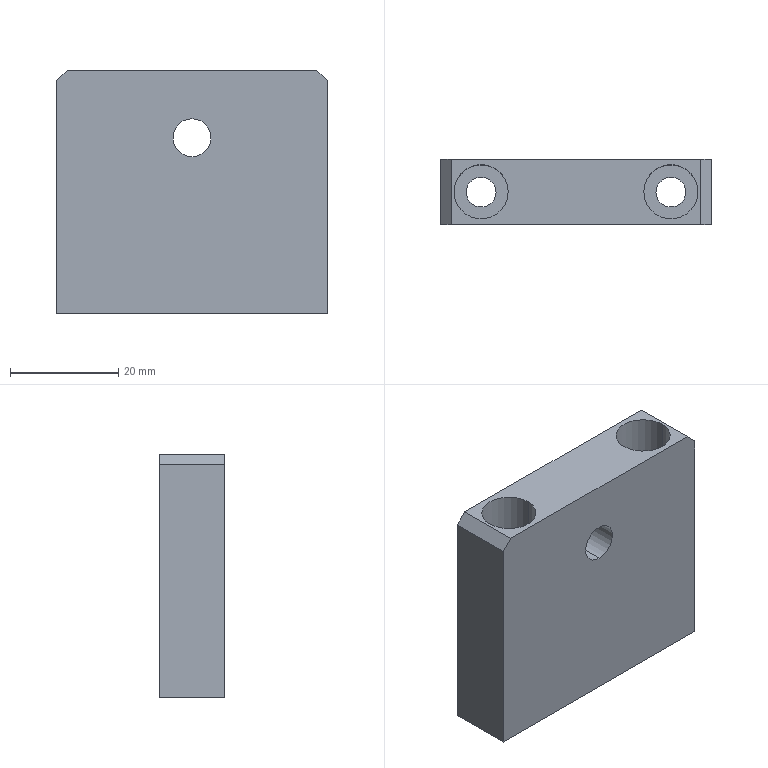Part | SolidWorks | features HoleWzd 2, Chamfer 1, Extrusion 1 | 1 solid | 20 faces | box 50 x 12 x 45 mm | volume 20517 mm3 | cylinder 10 | plane 10 | commonest cylinder face diameters 5.5 x4 10 x4 7 x2
STEP:
#1=CARTESIAN_POINT('',(-22.5,0.,-12.5));
#2=VERTEX_POINT('',#1);
#3=CARTESIAN_POINT('',(-12.5,0.,-12.5));
#4=VERTEX_POINT('',#3);
#5=CARTESIAN_POINT('',(-17.5,0.,-12.5));
#6=DIRECTION('',(0.,0.,1.));
#7=DIRECTION('',(1.,0.,0.));
#8=AXIS2_PLACEMENT_3D('',#5,#6,#7);
#9=CIRCLE('',#8,5.);
#10=EDGE_CURVE('',#2,#4,#9,.T.);
#11=ORIENTED_EDGE('',*,*,#10,.F.);
#12=CARTESIAN_POINT('',(-22.5,0.,22.5));
#13=VERTEX_POINT('',#12);
#14=CARTESIAN_POINT('',(-22.5,0.,22.5));
#15=DIRECTION('',(0.,0.,1.));
#16=VECTOR('',#15,1000.);
#17=LINE('',#14,#16);
#18=EDGE_CURVE('',#2,#13,#17,.T.);
#19=ORIENTED_EDGE('',*,*,#18,.T.);
#20=CARTESIAN_POINT('',(-12.5,0.,22.5));
#21=VERTEX_POINT('',#20);
#22=CARTESIAN_POINT('',(-17.5,0.,22.5));
#23=DIRECTION('',(0.,0.,1.));
#24=DIRECTION('',(1.,0.,0.));
#25=AXIS2_PLACEMENT_3D('',#22,#23,#24);
#26=CIRCLE('',#25,5.);
#27=EDGE_CURVE('',#13,#21,#26,.T.);
#28=ORIENTED_EDGE('',*,*,#27,.T.);
#29=CARTESIAN_POINT('',(-12.5,0.,22.5));
#30=DIRECTION('',(0.,0.,1.));
#31=VECTOR('',#30,1000.);
#32=LINE('',#29,#31);
#33=EDGE_CURVE('',#4,#21,#32,.T.);
#34=ORIENTED_EDGE('',*,*,#33,.F.);
#35=EDGE_LOOP('',(#11,#19,#28,#34));
#36=FACE_OUTER_BOUND('',#35,.T.);
#37=CARTESIAN_POINT('',(-17.5,0.,22.5));
#38=DIRECTION('',(0.,0.,1.));
#39=DIRECTION('',(1.,0.,0.));
#40=AXIS2_PLACEMENT_3D('',#37,#38,#39);
#41=CYLINDRICAL_SURFACE('',#40,5.);
#42=ADVANCED_FACE('',(#36),#41,.F.);
#43=CARTESIAN_POINT('',(-20.25,0.,-22.5));
#44=VERTEX_POINT('',#43);
#45=CARTESIAN_POINT('',(-14.75,0.,-22.5));
#46=VERTEX_POINT('',#45);
#47=CARTESIAN_POINT('',(-17.5,0.,-22.5));
#48=DIRECTION('',(0.,0.,1.));
#49=DIRECTION('',(1.,0.,0.));
#50=AXIS2_PLACEMENT_3D('',#47,#48,#49);
#51=CIRCLE('',#50,2.75);
#52=EDGE_CURVE('',#44,#46,#51,.T.);
#53=ORIENTED_EDGE('',*,*,#52,.F.);
#54=CARTESIAN_POINT('',(-20.25,0.,-12.5));
#55=VERTEX_POINT('',#54);
#56=CARTESIAN_POINT('',(-20.25,0.,22.5));
#57=DIRECTION('',(0.,0.,1.));
#58=VECTOR('',#57,1000.);
#59=LINE('',#56,#58);
#60=EDGE_CURVE('',#44,#55,#59,.T.);
#61=ORIENTED_EDGE('',*,*,#60,.T.);
#62=CARTESIAN_POINT('',(-14.75,0.,-12.5));
#63=VERTEX_POINT('',#62);
#64=CARTESIAN_POINT('',(-17.5,0.,-12.5));
#65=DIRECTION('',(0.,0.,1.));
#66=DIRECTION('',(1.,0.,0.));
#67=AXIS2_PLACEMENT_3D('',#64,#65,#66);
#68=CIRCLE('',#67,2.75);
#69=EDGE_CURVE('',#55,#63,#68,.T.);
#70=ORIENTED_EDGE('',*,*,#69,.T.);
#71=CARTESIAN_POINT('',(-14.75,0.,22.5));
#72=DIRECTION('',(0.,0.,1.));
#73=VECTOR('',#72,1000.);
#74=LINE('',#71,#73);
#75=EDGE_CURVE('',#46,#63,#74,.T.);
#76=ORIENTED_EDGE('',*,*,#75,.F.);
#77=EDGE_LOOP('',(#53,#61,#70,#76));
#78=FACE_OUTER_BOUND('',#77,.T.);
#79=CARTESIAN_POINT('',(-17.5,0.,22.5));
#80=DIRECTION('',(0.,0.,1.));
#81=DIRECTION('',(1.,0.,0.));
#82=AXIS2_PLACEMENT_3D('',#79,#80,#81);
#83=CYLINDRICAL_SURFACE('',#82,2.75);
#84=ADVANCED_FACE('',(#78),#83,.F.);
#85=CARTESIAN_POINT('',(12.5,0.,-12.5));
#86=VERTEX_POINT('',#85);
#87=CARTESIAN_POINT('',(22.5,0.,-12.5));
#88=VERTEX_POINT('',#87);
#89=CARTESIAN_POINT('',(17.5,0.,-12.5));
#90=DIRECTION('',(0.,0.,1.));
#91=DIRECTION('',(1.,0.,0.));
#92=AXIS2_PLACEMENT_3D('',#89,#90,#91);
#93=CIRCLE('',#92,5.);
#94=EDGE_CURVE('',#86,#88,#93,.T.);
#95=ORIENTED_EDGE('',*,*,#94,.F.);
#96=CARTESIAN_POINT('',(12.5,0.,22.5));
#97=VERTEX_POINT('',#96);
#98=CARTESIAN_POINT('',(12.5,0.,22.5));
#99=DIRECTION('',(0.,0.,1.));
#100=VECTOR('',#99,1000.);
#101=LINE('',#98,#100);
#102=EDGE_CURVE('',#86,#97,#101,.T.);
#103=ORIENTED_EDGE('',*,*,#102,.T.);
#104=CARTESIAN_POINT('',(22.5,0.,22.5));
#105=VERTEX_POINT('',#104);
#106=CARTESIAN_POINT('',(17.5,0.,22.5));
#107=DIRECTION('',(0.,0.,1.));
#108=DIRECTION('',(1.,0.,0.));
#109=AXIS2_PLACEMENT_3D('',#106,#107,#108);
#110=CIRCLE('',#109,5.);
#111=EDGE_CURVE('',#97,#105,#110,.T.);
#112=ORIENTED_EDGE('',*,*,#111,.T.);
#113=CARTESIAN_POINT('',(22.5,0.,22.5));
#114=DIRECTION('',(0.,0.,1.));
#115=VECTOR('',#114,1000.);
#116=LINE('',#113,#115);
#117=EDGE_CURVE('',#88,#105,#116,.T.);
#118=ORIENTED_EDGE('',*,*,#117,.F.);
#119=EDGE_LOOP('',(#95,#103,#112,#118));
#120=FACE_OUTER_BOUND('',#119,.T.);
#121=CARTESIAN_POINT('',(17.5,0.,22.5));
#122=DIRECTION('',(0.,0.,1.));
#123=DIRECTION('',(1.,0.,0.));
#124=AXIS2_PLACEMENT_3D('',#121,#122,#123);
#125=CYLINDRICAL_SURFACE('',#124,5.);
#126=ADVANCED_FACE('',(#120),#125,.F.);
#127=CARTESIAN_POINT('',(14.75,0.,-22.5));
#128=VERTEX_POINT('',#127);
#129=CARTESIAN_POINT('',(20.25,0.,-22.5));
#130=VERTEX_POINT('',#129);
#131=CARTESIAN_POINT('',(17.5,0.,-22.5));
#132=DIRECTION('',(0.,0.,1.));
#133=DIRECTION('',(1.,0.,0.));
#134=AXIS2_PLACEMENT_3D('',#131,#132,#133);
#135=CIRCLE('',#134,2.75);
#136=EDGE_CURVE('',#128,#130,#135,.T.);
#137=ORIENTED_EDGE('',*,*,#136,.F.);
#138=CARTESIAN_POINT('',(14.75,0.,-12.5));
#139=VERTEX_POINT('',#138);
#140=CARTESIAN_POINT('',(14.75,0.,22.5));
#141=DIRECTION('',(0.,0.,1.));
#142=VECTOR('',#141,1000.);
#143=LINE('',#140,#142);
#144=EDGE_CURVE('',#128,#139,#143,.T.);
#145=ORIENTED_EDGE('',*,*,#144,.T.);
#146=CARTESIAN_POINT('',(20.25,0.,-12.5));
#147=VERTEX_POINT('',#146);
#148=CARTESIAN_POINT('',(17.5,0.,-12.5));
#149=DIRECTION('',(0.,0.,1.));
#150=DIRECTION('',(1.,0.,0.));
#151=AXIS2_PLACEMENT_3D('',#148,#149,#150);
#152=CIRCLE('',#151,2.75);
#153=EDGE_CURVE('',#139,#147,#152,.T.);
#154=ORIENTED_EDGE('',*,*,#153,.T.);
#155=CARTESIAN_POINT('',(20.25,0.,22.5));
#156=DIRECTION('',(0.,0.,1.));
#157=VECTOR('',#156,1000.);
#158=LINE('',#155,#157);
#159=EDGE_CURVE('',#130,#147,#158,.T.);
#160=ORIENTED_EDGE('',*,*,#159,.F.);
#161=EDGE_LOOP('',(#137,#145,#154,#160));
#162=FACE_OUTER_BOUND('',#161,.T.);
#163=CARTESIAN_POINT('',(17.5,0.,22.5));
#164=DIRECTION('',(0.,0.,1.));
#165=DIRECTION('',(1.,0.,0.));
#166=AXIS2_PLACEMENT_3D('',#163,#164,#165);
#167=CYLINDRICAL_SURFACE('',#166,2.75);
#168=ADVANCED_FACE('',(#162),#167,.F.);
#169=CARTESIAN_POINT('',(0.,-6.,6.5));
#170=VERTEX_POINT('',#169);
#171=CARTESIAN_POINT('',(0.,-6.,13.5));
#172=VERTEX_POINT('',#171);
#173=CARTESIAN_POINT('',(0.,-6.,10.));
#174=DIRECTION('',(0.,1.,0.));
#175=DIRECTION('',(-1.,0.,0.));
#176=AXIS2_PLACEMENT_3D('',#173,#174,#175);
#177=CIRCLE('',#176,3.5);
#178=EDGE_CURVE('',#170,#172,#177,.T.);
#179=ORIENTED_EDGE('',*,*,#178,.F.);
#180=CARTESIAN_POINT('',(0.,6.,6.5));
#181=VERTEX_POINT('',#180);
#182=CARTESIAN_POINT('',(0.,6.,6.5));
#183=DIRECTION('',(0.,1.,0.));
#184=VECTOR('',#183,1000.);
#185=LINE('',#182,#184);
#186=EDGE_CURVE('',#170,#181,#185,.T.);
#187=ORIENTED_EDGE('',*,*,#186,.T.);
#188=CARTESIAN_POINT('',(0.,6.,13.5));
#189=VERTEX_POINT('',#188);
#190=CARTESIAN_POINT('',(0.,6.,10.));
#191=DIRECTION('',(0.,1.,0.));
#192=DIRECTION('',(0.,0.,1.));
#193=AXIS2_PLACEMENT_3D('',#190,#191,#192);
#194=CIRCLE('',#193,3.5);
#195=EDGE_CURVE('',#181,#189,#194,.T.);
#196=ORIENTED_EDGE('',*,*,#195,.T.);
#197=CARTESIAN_POINT('',(0.,6.,13.5));
#198=DIRECTION('',(0.,1.,0.));
#199=VECTOR('',#198,1000.);
#200=LINE('',#197,#199);
#201=EDGE_CURVE('',#172,#189,#200,.T.);
#202=ORIENTED_EDGE('',*,*,#201,.F.);
#203=EDGE_LOOP('',(#179,#187,#196,#202));
#204=FACE_OUTER_BOUND('',#203,.T.);
#205=CARTESIAN_POINT('',(0.,6.,10.));
#206=DIRECTION('',(0.,1.,0.));
#207=DIRECTION('',(0.,0.,1.));
#208=AXIS2_PLACEMENT_3D('',#205,#206,#207);
#209=CYLINDRICAL_SURFACE('',#208,3.5);
#210=ADVANCED_FACE('',(#204),#209,.F.);
#211=CARTESIAN_POINT('',(-25.,6.,20.5));
#212=VERTEX_POINT('',#211);
#213=CARTESIAN_POINT('',(-25.,6.,-22.5));
#214=VERTEX_POINT('',#213);
#215=CARTESIAN_POINT('',(-25.,6.,22.5));
#216=DIRECTION('',(0.,0.,-1.));
#217=VECTOR('',#216,1000.);
#218=LINE('',#215,#217);
#219=EDGE_CURVE('',#212,#214,#218,.T.);
#220=ORIENTED_EDGE('',*,*,#219,.F.);
#221=CARTESIAN_POINT('',(-23.,6.,22.5));
#222=VERTEX_POINT('',#221);
#223=CARTESIAN_POINT('',(-23.,6.,22.5));
#224=DIRECTION('',(0.7071,0.,0.7071));
#225=VECTOR('',#224,1000.);
#226=LINE('',#223,#225);
#227=EDGE_CURVE('',#212,#222,#226,.T.);
#228=ORIENTED_EDGE('',*,*,#227,.T.);
#229=CARTESIAN_POINT('',(23.,6.,22.5));
#230=VERTEX_POINT('',#229);
#231=CARTESIAN_POINT('',(25.,6.,22.5));
#232=DIRECTION('',(-1.,0.,0.));
#233=VECTOR('',#232,1000.);
#234=LINE('',#231,#233);
#235=EDGE_CURVE('',#230,#222,#234,.T.);
#236=ORIENTED_EDGE('',*,*,#235,.F.);
#237=CARTESIAN_POINT('',(25.,6.,20.5));
#238=VERTEX_POINT('',#237);
#239=CARTESIAN_POINT('',(23.,6.,22.5));
#240=DIRECTION('',(0.7071,0.,-0.7071));
#241=VECTOR('',#240,1000.);
#242=LINE('',#239,#241);
#243=EDGE_CURVE('',#230,#238,#242,.T.);
#244=ORIENTED_EDGE('',*,*,#243,.T.);
#245=CARTESIAN_POINT('',(25.,6.,-22.5));
#246=VERTEX_POINT('',#245);
#247=CARTESIAN_POINT('',(25.,6.,22.5));
#248=DIRECTION('',(0.,0.,-1.));
#249=VECTOR('',#248,1000.);
#250=LINE('',#247,#249);
#251=EDGE_CURVE('',#238,#246,#250,.T.);
#252=ORIENTED_EDGE('',*,*,#251,.T.);
#253=CARTESIAN_POINT('',(25.,6.,-22.5));
#254=DIRECTION('',(-1.,0.,0.));
#255=VECTOR('',#254,1000.);
#256=LINE('',#253,#255);
#257=EDGE_CURVE('',#246,#214,#256,.T.);
#258=ORIENTED_EDGE('',*,*,#257,.T.);
#259=EDGE_LOOP('',(#220,#228,#236,#244,#252,#258));
#260=FACE_OUTER_BOUND('',#259,.T.);
#261=CARTESIAN_POINT('',(0.,6.,10.));
#262=DIRECTION('',(0.,1.,0.));
#263=DIRECTION('',(0.,0.,1.));
#264=AXIS2_PLACEMENT_3D('',#261,#262,#263);
#265=CIRCLE('',#264,3.5);
#266=EDGE_CURVE('',#189,#181,#265,.T.);
#267=ORIENTED_EDGE('',*,*,#266,.F.);
#268=ORIENTED_EDGE('',*,*,#195,.F.);
#269=EDGE_LOOP('',(#267,#268));
#270=FACE_BOUND('',#269,.T.);
#271=CARTESIAN_POINT('',(25.,6.,22.5));
#272=DIRECTION('',(0.,-1.,0.));
#273=DIRECTION('',(1.,0.,0.));
#274=AXIS2_PLACEMENT_3D('',#271,#272,#273);
#275=PLANE('',#274);
#276=ADVANCED_FACE('',(#260,#270),#275,.F.);
#277=CARTESIAN_POINT('',(-25.,-6.,20.5));
#278=VERTEX_POINT('',#277);
#279=CARTESIAN_POINT('',(-25.,-6.,-22.5));
#280=VERTEX_POINT('',#279);
#281=CARTESIAN_POINT('',(-25.,-6.,22.5));
#282=DIRECTION('',(0.,0.,-1.));
#283=VECTOR('',#282,1000.);
#284=LINE('',#281,#283);
#285=EDGE_CURVE('',#278,#280,#284,.T.);
#286=ORIENTED_EDGE('',*,*,#285,.F.);
#287=CARTESIAN_POINT('',(-25.,6.,20.5));
#288=DIRECTION('',(0.,1.,0.));
#289=VECTOR('',#288,1000.);
#290=LINE('',#287,#289);
#291=EDGE_CURVE('',#278,#212,#290,.T.);
#292=ORIENTED_EDGE('',*,*,#291,.T.);
#293=ORIENTED_EDGE('',*,*,#219,.T.);
#294=CARTESIAN_POINT('',(-25.,-6.,-22.5));
#295=DIRECTION('',(0.,-1.,0.));
#296=VECTOR('',#295,1000.);
#297=LINE('',#294,#296);
#298=EDGE_CURVE('',#214,#280,#297,.T.);
#299=ORIENTED_EDGE('',*,*,#298,.T.);
#300=EDGE_LOOP('',(#286,#292,#293,#299));
#301=FACE_OUTER_BOUND('',#300,.T.);
#302=CARTESIAN_POINT('',(-25.,-6.,22.5));
#303=DIRECTION('',(1.,0.,0.));
#304=DIRECTION('',(0.,0.,-1.));
#305=AXIS2_PLACEMENT_3D('',#302,#303,#304);
#306=PLANE('',#305);
#307=ADVANCED_FACE('',(#301),#306,.F.);
#308=CARTESIAN_POINT('',(0.,-6.,10.));
#309=DIRECTION('',(0.,1.,0.));
#310=DIRECTION('',(-1.,0.,0.));
#311=AXIS2_PLACEMENT_3D('',#308,#309,#310);
#312=CIRCLE('',#311,3.5);
#313=EDGE_CURVE('',#172,#170,#312,.T.);
#314=ORIENTED_EDGE('',*,*,#313,.T.);
#315=ORIENTED_EDGE('',*,*,#178,.T.);
#316=EDGE_LOOP('',(#314,#315));
#317=FACE_BOUND('',#316,.T.);
#318=CARTESIAN_POINT('',(-23.,-6.,22.5));
#319=VERTEX_POINT('',#318);
#320=CARTESIAN_POINT('',(23.,-6.,22.5));
#321=VERTEX_POINT('',#320);
#322=CARTESIAN_POINT('',(25.,-6.,22.5));
#323=DIRECTION('',(1.,0.,0.));
#324=VECTOR('',#323,1000.);
#325=LINE('',#322,#324);
#326=EDGE_CURVE('',#319,#321,#325,.T.);
#327=ORIENTED_EDGE('',*,*,#326,.F.);
#328=CARTESIAN_POINT('',(-23.,-6.,22.5));
#329=DIRECTION('',(-0.7071,0.,-0.7071));
#330=VECTOR('',#329,1000.);
#331=LINE('',#328,#330);
#332=EDGE_CURVE('',#319,#278,#331,.T.);
#333=ORIENTED_EDGE('',*,*,#332,.T.);
#334=ORIENTED_EDGE('',*,*,#285,.T.);
#335=CARTESIAN_POINT('',(25.,-6.,-22.5));
#336=VERTEX_POINT('',#335);
#337=CARTESIAN_POINT('',(25.,-6.,-22.5));
#338=DIRECTION('',(1.,0.,0.));
#339=VECTOR('',#338,1000.);
#340=LINE('',#337,#339);
#341=EDGE_CURVE('',#280,#336,#340,.T.);
#342=ORIENTED_EDGE('',*,*,#341,.T.);
#343=CARTESIAN_POINT('',(25.,-6.,20.5));
#344=VERTEX_POINT('',#343);
#345=CARTESIAN_POINT('',(25.,-6.,22.5));
#346=DIRECTION('',(0.,0.,-1.));
#347=VECTOR('',#346,1000.);
#348=LINE('',#345,#347);
#349=EDGE_CURVE('',#344,#336,#348,.T.);
#350=ORIENTED_EDGE('',*,*,#349,.F.);
#351=CARTESIAN_POINT('',(23.,-6.,22.5));
#352=DIRECTION('',(-0.7071,0.,0.7071));
#353=VECTOR('',#352,1000.);
#354=LINE('',#351,#353);
#355=EDGE_CURVE('',#344,#321,#354,.T.);
#356=ORIENTED_EDGE('',*,*,#355,.T.);
#357=EDGE_LOOP('',(#327,#333,#334,#342,#350,#356));
#358=FACE_OUTER_BOUND('',#357,.T.);
#359=CARTESIAN_POINT('',(25.,-6.,22.5));
#360=DIRECTION('',(0.,1.,0.));
#361=DIRECTION('',(-1.,0.,0.));
#362=AXIS2_PLACEMENT_3D('',#359,#360,#361);
#363=PLANE('',#362);
#364=ADVANCED_FACE('',(#317,#358),#363,.F.);
#365=ORIENTED_EDGE('',*,*,#251,.F.);
#366=CARTESIAN_POINT('',(25.,-6.,20.5));
#367=DIRECTION('',(0.,-1.,0.));
#368=VECTOR('',#367,1000.);
#369=LINE('',#366,#368);
#370=EDGE_CURVE('',#238,#344,#369,.T.);
#371=ORIENTED_EDGE('',*,*,#370,.T.);
#372=ORIENTED_EDGE('',*,*,#349,.T.);
#373=CARTESIAN_POINT('',(25.,-6.,-22.5));
#374=DIRECTION('',(0.,1.,0.));
#375=VECTOR('',#374,1000.);
#376=LINE('',#373,#375);
#377=EDGE_CURVE('',#336,#246,#376,.T.);
#378=ORIENTED_EDGE('',*,*,#377,.T.);
#379=EDGE_LOOP('',(#365,#371,#372,#378));
#380=FACE_OUTER_BOUND('',#379,.T.);
#381=CARTESIAN_POINT('',(25.,-6.,22.5));
#382=DIRECTION('',(-1.,0.,0.));
#383=DIRECTION('',(0.,0.,1.));
#384=AXIS2_PLACEMENT_3D('',#381,#382,#383);
#385=PLANE('',#384);
#386=ADVANCED_FACE('',(#380),#385,.F.);
#387=CARTESIAN_POINT('',(-17.5,0.,22.5));
#388=DIRECTION('',(0.,0.,1.));
#389=DIRECTION('',(1.,0.,0.));
#390=AXIS2_PLACEMENT_3D('',#387,#388,#389);
#391=CIRCLE('',#390,5.);
#392=EDGE_CURVE('',#21,#13,#391,.T.);
#393=ORIENTED_EDGE('',*,*,#392,.F.);
#394=ORIENTED_EDGE('',*,*,#27,.F.);
#395=EDGE_LOOP('',(#393,#394));
#396=FACE_BOUND('',#395,.T.);
#397=CARTESIAN_POINT('',(17.5,0.,22.5));
#398=DIRECTION('',(0.,0.,1.));
#399=DIRECTION('',(1.,0.,0.));
#400=AXIS2_PLACEMENT_3D('',#397,#398,#399);
#401=CIRCLE('',#400,5.);
#402=EDGE_CURVE('',#105,#97,#401,.T.);
#403=ORIENTED_EDGE('',*,*,#402,.F.);
#404=ORIENTED_EDGE('',*,*,#111,.F.);
#405=EDGE_LOOP('',(#403,#404));
#406=FACE_BOUND('',#405,.T.);
#407=ORIENTED_EDGE('',*,*,#235,.T.);
#408=CARTESIAN_POINT('',(-23.,-6.,22.5));
#409=DIRECTION('',(0.,-1.,0.));
#410=VECTOR('',#409,1000.);
#411=LINE('',#408,#410);
#412=EDGE_CURVE('',#222,#319,#411,.T.);
#413=ORIENTED_EDGE('',*,*,#412,.T.);
#414=ORIENTED_EDGE('',*,*,#326,.T.);
#415=CARTESIAN_POINT('',(23.,6.,22.5));
#416=DIRECTION('',(0.,1.,0.));
#417=VECTOR('',#416,1000.);
#418=LINE('',#415,#417);
#419=EDGE_CURVE('',#321,#230,#418,.T.);
#420=ORIENTED_EDGE('',*,*,#419,.T.);
#421=EDGE_LOOP('',(#407,#413,#414,#420));
#422=FACE_OUTER_BOUND('',#421,.T.);
#423=CARTESIAN_POINT('',(0.,0.,22.5));
#424=DIRECTION('',(0.,0.,1.));
#425=DIRECTION('',(1.,0.,0.));
#426=AXIS2_PLACEMENT_3D('',#423,#424,#425);
#427=PLANE('',#426);
#428=ADVANCED_FACE('',(#396,#406,#422),#427,.T.);
#429=CARTESIAN_POINT('',(-17.5,0.,-22.5));
#430=DIRECTION('',(0.,0.,1.));
#431=DIRECTION('',(1.,0.,0.));
#432=AXIS2_PLACEMENT_3D('',#429,#430,#431);
#433=CIRCLE('',#432,2.75);
#434=EDGE_CURVE('',#46,#44,#433,.T.);
#435=ORIENTED_EDGE('',*,*,#434,.T.);
#436=ORIENTED_EDGE('',*,*,#52,.T.);
#437=EDGE_LOOP('',(#435,#436));
#438=FACE_BOUND('',#437,.T.);
#439=CARTESIAN_POINT('',(17.5,0.,-22.5));
#440=DIRECTION('',(0.,0.,1.));
#441=DIRECTION('',(1.,0.,0.));
#442=AXIS2_PLACEMENT_3D('',#439,#440,#441);
#443=CIRCLE('',#442,2.75);
#444=EDGE_CURVE('',#130,#128,#443,.T.);
#445=ORIENTED_EDGE('',*,*,#444,.T.);
#446=ORIENTED_EDGE('',*,*,#136,.T.);
#447=EDGE_LOOP('',(#445,#446));
#448=FACE_BOUND('',#447,.T.);
#449=ORIENTED_EDGE('',*,*,#298,.F.);
#450=ORIENTED_EDGE('',*,*,#257,.F.);
#451=ORIENTED_EDGE('',*,*,#377,.F.);
#452=ORIENTED_EDGE('',*,*,#341,.F.);
#453=EDGE_LOOP('',(#449,#450,#451,#452));
#454=FACE_OUTER_BOUND('',#453,.T.);
#455=CARTESIAN_POINT('',(0.,0.,-22.5));
#456=DIRECTION('',(0.,0.,1.));
#457=DIRECTION('',(1.,0.,0.));
#458=AXIS2_PLACEMENT_3D('',#455,#456,#457);
#459=PLANE('',#458);
#460=ADVANCED_FACE('',(#438,#448,#454),#459,.F.);
#461=ORIENTED_EDGE('',*,*,#186,.F.);
#462=ORIENTED_EDGE('',*,*,#313,.F.);
#463=ORIENTED_EDGE('',*,*,#201,.T.);
#464=ORIENTED_EDGE('',*,*,#266,.T.);
#465=EDGE_LOOP('',(#461,#462,#463,#464));
#466=FACE_OUTER_BOUND('',#465,.T.);
#467=CARTESIAN_POINT('',(0.,6.,10.));
#468=DIRECTION('',(0.,1.,0.));
#469=DIRECTION('',(0.,0.,1.));
#470=AXIS2_PLACEMENT_3D('',#467,#468,#469);
#471=CYLINDRICAL_SURFACE('',#470,3.5);
#472=ADVANCED_FACE('',(#466),#471,.F.);
#473=ORIENTED_EDGE('',*,*,#144,.F.);
#474=ORIENTED_EDGE('',*,*,#444,.F.);
#475=ORIENTED_EDGE('',*,*,#159,.T.);
#476=CARTESIAN_POINT('',(17.5,0.,-12.5));
#477=DIRECTION('',(0.,0.,1.));
#478=DIRECTION('',(1.,0.,0.));
#479=AXIS2_PLACEMENT_3D('',#476,#477,#478);
#480=CIRCLE('',#479,2.75);
#481=EDGE_CURVE('',#147,#139,#480,.T.);
#482=ORIENTED_EDGE('',*,*,#481,.T.);
#483=EDGE_LOOP('',(#473,#474,#475,#482));
#484=FACE_OUTER_BOUND('',#483,.T.);
#485=CARTESIAN_POINT('',(17.5,0.,22.5));
#486=DIRECTION('',(0.,0.,1.));
#487=DIRECTION('',(1.,0.,0.));
#488=AXIS2_PLACEMENT_3D('',#485,#486,#487);
#489=CYLINDRICAL_SURFACE('',#488,2.75);
#490=ADVANCED_FACE('',(#484),#489,.F.);
#491=ORIENTED_EDGE('',*,*,#481,.F.);
#492=ORIENTED_EDGE('',*,*,#153,.F.);
#493=EDGE_LOOP('',(#491,#492));
#494=FACE_BOUND('',#493,.T.);
#495=CARTESIAN_POINT('',(17.5,0.,-12.5));
#496=DIRECTION('',(0.,0.,1.));
#497=DIRECTION('',(1.,0.,0.));
#498=AXIS2_PLACEMENT_3D('',#495,#496,#497);
#499=CIRCLE('',#498,5.);
#500=EDGE_CURVE('',#88,#86,#499,.T.);
#501=ORIENTED_EDGE('',*,*,#500,.T.);
#502=ORIENTED_EDGE('',*,*,#94,.T.);
#503=EDGE_LOOP('',(#501,#502));
#504=FACE_OUTER_BOUND('',#503,.T.);
#505=CARTESIAN_POINT('',(20.25,0.,-12.5));
#506=DIRECTION('',(0.,0.,-1.));
#507=DIRECTION('',(-1.,0.,0.));
#508=AXIS2_PLACEMENT_3D('',#505,#506,#507);
#509=PLANE('',#508);
#510=ADVANCED_FACE('',(#494,#504),#509,.F.);
#511=ORIENTED_EDGE('',*,*,#102,.F.);
#512=ORIENTED_EDGE('',*,*,#500,.F.);
#513=ORIENTED_EDGE('',*,*,#117,.T.);
#514=ORIENTED_EDGE('',*,*,#402,.T.);
#515=EDGE_LOOP('',(#511,#512,#513,#514));
#516=FACE_OUTER_BOUND('',#515,.T.);
#517=CARTESIAN_POINT('',(17.5,0.,22.5));
#518=DIRECTION('',(0.,0.,1.));
#519=DIRECTION('',(1.,0.,0.));
#520=AXIS2_PLACEMENT_3D('',#517,#518,#519);
#521=CYLINDRICAL_SURFACE('',#520,5.);
#522=ADVANCED_FACE('',(#516),#521,.F.);
#523=ORIENTED_EDGE('',*,*,#60,.F.);
#524=ORIENTED_EDGE('',*,*,#434,.F.);
#525=ORIENTED_EDGE('',*,*,#75,.T.);
#526=CARTESIAN_POINT('',(-17.5,0.,-12.5));
#527=DIRECTION('',(0.,0.,1.));
#528=DIRECTION('',(1.,0.,0.));
#529=AXIS2_PLACEMENT_3D('',#526,#527,#528);
#530=CIRCLE('',#529,2.75);
#531=EDGE_CURVE('',#63,#55,#530,.T.);
#532=ORIENTED_EDGE('',*,*,#531,.T.);
#533=EDGE_LOOP('',(#523,#524,#525,#532));
#534=FACE_OUTER_BOUND('',#533,.T.);
#535=CARTESIAN_POINT('',(-17.5,0.,22.5));
#536=DIRECTION('',(0.,0.,1.));
#537=DIRECTION('',(1.,0.,0.));
#538=AXIS2_PLACEMENT_3D('',#535,#536,#537);
#539=CYLINDRICAL_SURFACE('',#538,2.75);
#540=ADVANCED_FACE('',(#534),#539,.F.);
#541=ORIENTED_EDGE('',*,*,#531,.F.);
#542=ORIENTED_EDGE('',*,*,#69,.F.);
#543=EDGE_LOOP('',(#541,#542));
#544=FACE_BOUND('',#543,.T.);
#545=CARTESIAN_POINT('',(-17.5,0.,-12.5));
#546=DIRECTION('',(0.,0.,1.));
#547=DIRECTION('',(1.,0.,0.));
#548=AXIS2_PLACEMENT_3D('',#545,#546,#547);
#549=CIRCLE('',#548,5.);
#550=EDGE_CURVE('',#4,#2,#549,.T.);
#551=ORIENTED_EDGE('',*,*,#550,.T.);
#552=ORIENTED_EDGE('',*,*,#10,.T.);
#553=EDGE_LOOP('',(#551,#552));
#554=FACE_OUTER_BOUND('',#553,.T.);
#555=CARTESIAN_POINT('',(-14.75,0.,-12.5));
#556=DIRECTION('',(0.,0.,-1.));
#557=DIRECTION('',(-1.,0.,0.));
#558=AXIS2_PLACEMENT_3D('',#555,#556,#557);
#559=PLANE('',#558);
#560=ADVANCED_FACE('',(#544,#554),#559,.F.);
#561=ORIENTED_EDGE('',*,*,#18,.F.);
#562=ORIENTED_EDGE('',*,*,#550,.F.);
#563=ORIENTED_EDGE('',*,*,#33,.T.);
#564=ORIENTED_EDGE('',*,*,#392,.T.);
#565=EDGE_LOOP('',(#561,#562,#563,#564));
#566=FACE_OUTER_BOUND('',#565,.T.);
#567=CARTESIAN_POINT('',(-17.5,0.,22.5));
#568=DIRECTION('',(0.,0.,1.));
#569=DIRECTION('',(1.,0.,0.));
#570=AXIS2_PLACEMENT_3D('',#567,#568,#569);
#571=CYLINDRICAL_SURFACE('',#570,5.);
#572=ADVANCED_FACE('',(#566),#571,.F.);
#573=ORIENTED_EDGE('',*,*,#227,.F.);
#574=ORIENTED_EDGE('',*,*,#291,.F.);
#575=ORIENTED_EDGE('',*,*,#332,.F.);
#576=ORIENTED_EDGE('',*,*,#412,.F.);
#577=EDGE_LOOP('',(#573,#574,#575,#576));
#578=FACE_OUTER_BOUND('',#577,.T.);
#579=CARTESIAN_POINT('',(-23.,0.,22.5));
#580=DIRECTION('',(-0.7071,0.,0.7071));
#581=DIRECTION('',(0.,1.,0.));
#582=AXIS2_PLACEMENT_3D('',#579,#580,#581);
#583=PLANE('',#582);
#584=ADVANCED_FACE('',(#578),#583,.T.);
#585=ORIENTED_EDGE('',*,*,#355,.F.);
#586=ORIENTED_EDGE('',*,*,#370,.F.);
#587=ORIENTED_EDGE('',*,*,#243,.F.);
#588=ORIENTED_EDGE('',*,*,#419,.F.);
#589=EDGE_LOOP('',(#585,#586,#587,#588));
#590=FACE_OUTER_BOUND('',#589,.T.);
#591=CARTESIAN_POINT('',(23.,0.,22.5));
#592=DIRECTION('',(0.7071,0.,0.7071));
#593=DIRECTION('',(0.,-1.,0.));
#594=AXIS2_PLACEMENT_3D('',#591,#592,#593);
#595=PLANE('',#594);
#596=ADVANCED_FACE('',(#590),#595,.T.);
#597=CLOSED_SHELL('',(#42,#84,#126,#168,#210,#276,#307,#364,#386,#428,#460,#472,#490,#510,#522,#540,#560,#572,#584,#596));
#598=MANIFOLD_SOLID_BREP('',#597);
#599=CARTESIAN_POINT('',(0.,0.,0.));
#600=DIRECTION('',(0.,0.,1.));
#601=DIRECTION('',(1.,0.,0.));
#602=AXIS2_PLACEMENT_3D('',#599,#600,#601);
#603=(LENGTH_UNIT()NAMED_UNIT(*)SI_UNIT(.MILLI.,.METRE.));
#604=UNCERTAINTY_MEASURE_WITH_UNIT(LENGTH_MEASURE(0.00001),#603,'','');
#605=(NAMED_UNIT(*)PLANE_ANGLE_UNIT()SI_UNIT($,.RADIAN.));
#606=(NAMED_UNIT(*)SI_UNIT($,.STERADIAN.)SOLID_ANGLE_UNIT());
#607=(GEOMETRIC_REPRESENTATION_CONTEXT(3)GLOBAL_UNCERTAINTY_ASSIGNED_CONTEXT((#604))GLOBAL_UNIT_ASSIGNED_CONTEXT((#603,#605,#606))REPRESENTATION_CONTEXT('',''));
#608=ADVANCED_BREP_SHAPE_REPRESENTATION('',(#598,#602),#607);